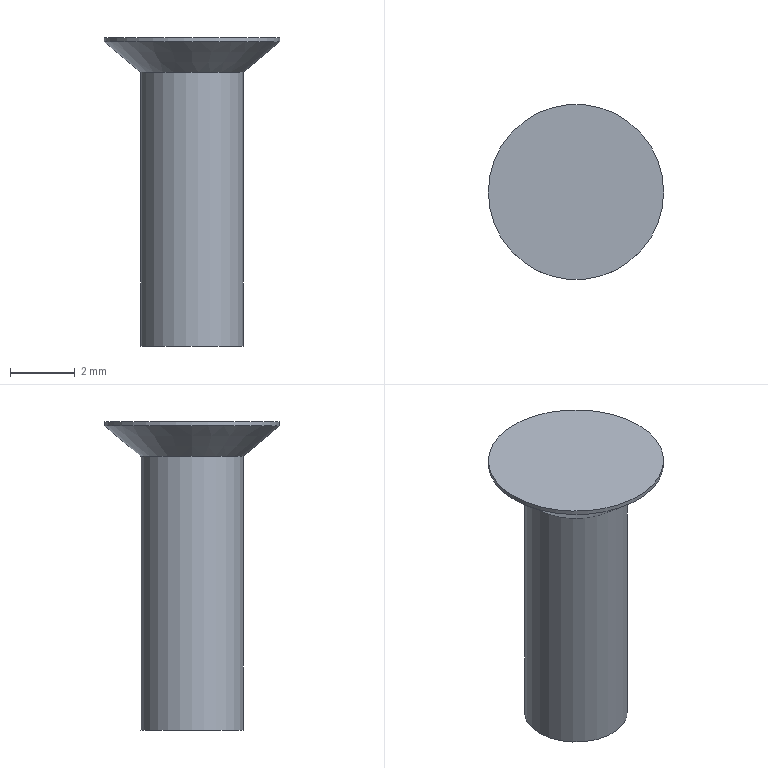Part | NX | features solid 2 | 1 solid | 5 faces | box 5.412 x 5.412 x 9.525 mm | volume 83.795 mm3 | cylinder 2 | plane 2 | cone 1 | commonest cylinder face diameters 3.175 x1 5.412 x1
STEP:
#1=CARTESIAN_POINT('',(-2.706,0.,-0.127));
#2=VERTEX_POINT('',#1);
#3=CARTESIAN_POINT('',(0.,0.,-0.127));
#4=DIRECTION('',(0.,0.,-1.));
#5=DIRECTION('',(-1.,0.,0.));
#6=AXIS2_PLACEMENT_3D('',#3,#4,#5);
#7=CIRCLE('',#6,2.706);
#8=EDGE_CURVE('',#2,#2,#7,.T.);
#9=ORIENTED_EDGE('',*,*,#8,.T.);
#10=EDGE_LOOP('',(#9));
#11=FACE_BOUND('',#10,.T.);
#12=CARTESIAN_POINT('',(-1.587,0.,-1.066));
#13=VERTEX_POINT('',#12);
#14=CARTESIAN_POINT('',(0.,0.,-1.066));
#15=DIRECTION('',(0.,0.,-1.));
#16=DIRECTION('',(-1.,0.,0.));
#17=AXIS2_PLACEMENT_3D('',#14,#15,#16);
#18=CIRCLE('',#17,1.587);
#19=EDGE_CURVE('',#13,#13,#18,.T.);
#20=ORIENTED_EDGE('',*,*,#19,.F.);
#21=EDGE_LOOP('',(#20));
#22=FACE_BOUND('',#21,.T.);
#23=CARTESIAN_POINT('',(0.,0.,-1.066));
#24=DIRECTION('',(0.,0.,1.));
#25=DIRECTION('',(1.,0.,0.));
#26=AXIS2_PLACEMENT_3D('',#23,#24,#25);
#27=CONICAL_SURFACE('',#26,1.587,0.8727);
#28=ADVANCED_FACE('',(#11,#22),#27,.T.);
#29=CARTESIAN_POINT('',(-2.706,0.,0.));
#30=VERTEX_POINT('',#29);
#31=CARTESIAN_POINT('',(0.,0.,0.));
#32=DIRECTION('',(0.,0.,-1.));
#33=DIRECTION('',(-1.,0.,0.));
#34=AXIS2_PLACEMENT_3D('',#31,#32,#33);
#35=CIRCLE('',#34,2.706);
#36=EDGE_CURVE('',#30,#30,#35,.T.);
#37=ORIENTED_EDGE('',*,*,#36,.T.);
#38=EDGE_LOOP('',(#37));
#39=FACE_BOUND('',#38,.T.);
#40=ORIENTED_EDGE('',*,*,#8,.F.);
#41=EDGE_LOOP('',(#40));
#42=FACE_BOUND('',#41,.T.);
#43=CARTESIAN_POINT('',(0.,0.,0.));
#44=DIRECTION('',(0.,0.,-1.));
#45=DIRECTION('',(-1.,0.,0.));
#46=AXIS2_PLACEMENT_3D('',#43,#44,#45);
#47=CYLINDRICAL_SURFACE('',#46,2.706);
#48=ADVANCED_FACE('',(#39,#42),#47,.T.);
#49=ORIENTED_EDGE('',*,*,#36,.F.);
#50=EDGE_LOOP('',(#49));
#51=FACE_BOUND('',#50,.T.);
#52=CARTESIAN_POINT('',(2.706,0.,0.));
#53=DIRECTION('',(0.,0.,1.));
#54=DIRECTION('',(1.,0.,0.));
#55=AXIS2_PLACEMENT_3D('',#52,#53,#54);
#56=PLANE('',#55);
#57=ADVANCED_FACE('',(#51),#56,.T.);
#58=CARTESIAN_POINT('',(-1.587,0.,-9.525));
#59=VERTEX_POINT('',#58);
#60=CARTESIAN_POINT('',(0.,0.,-9.525));
#61=DIRECTION('',(0.,0.,-1.));
#62=DIRECTION('',(-1.,0.,0.));
#63=AXIS2_PLACEMENT_3D('',#60,#61,#62);
#64=CIRCLE('',#63,1.587);
#65=EDGE_CURVE('',#59,#59,#64,.T.);
#66=ORIENTED_EDGE('',*,*,#65,.T.);
#67=EDGE_LOOP('',(#66));
#68=FACE_BOUND('',#67,.T.);
#69=CARTESIAN_POINT('',(0.,0.,-9.525));
#70=DIRECTION('',(0.,0.,-1.));
#71=DIRECTION('',(-1.,0.,0.));
#72=AXIS2_PLACEMENT_3D('',#69,#70,#71);
#73=PLANE('',#72);
#74=ADVANCED_FACE('',(#68),#73,.T.);
#75=ORIENTED_EDGE('',*,*,#19,.T.);
#76=EDGE_LOOP('',(#75));
#77=FACE_BOUND('',#76,.T.);
#78=ORIENTED_EDGE('',*,*,#65,.F.);
#79=EDGE_LOOP('',(#78));
#80=FACE_BOUND('',#79,.T.);
#81=CARTESIAN_POINT('',(0.,0.,0.));
#82=DIRECTION('',(0.,0.,-1.));
#83=DIRECTION('',(-1.,0.,0.));
#84=AXIS2_PLACEMENT_3D('',#81,#82,#83);
#85=CYLINDRICAL_SURFACE('',#84,1.587);
#86=ADVANCED_FACE('',(#77,#80),#85,.T.);
#87=CLOSED_SHELL('',(#28,#48,#57,#74,#86));
#88=MANIFOLD_SOLID_BREP('',#87);
#89=(LENGTH_UNIT()NAMED_UNIT(*)SI_UNIT(.MILLI.,.METRE.));
#90=UNCERTAINTY_MEASURE_WITH_UNIT(LENGTH_MEASURE(0.00001),#89,'','');
#91=(NAMED_UNIT(*)PLANE_ANGLE_UNIT()SI_UNIT($,.RADIAN.));
#92=(NAMED_UNIT(*)SI_UNIT($,.STERADIAN.)SOLID_ANGLE_UNIT());
#93=(GEOMETRIC_REPRESENTATION_CONTEXT(3)GLOBAL_UNCERTAINTY_ASSIGNED_CONTEXT((#90))GLOBAL_UNIT_ASSIGNED_CONTEXT((#89,#91,#92))REPRESENTATION_CONTEXT('',''));
#94=ADVANCED_BREP_SHAPE_REPRESENTATION('',(#88),#93);